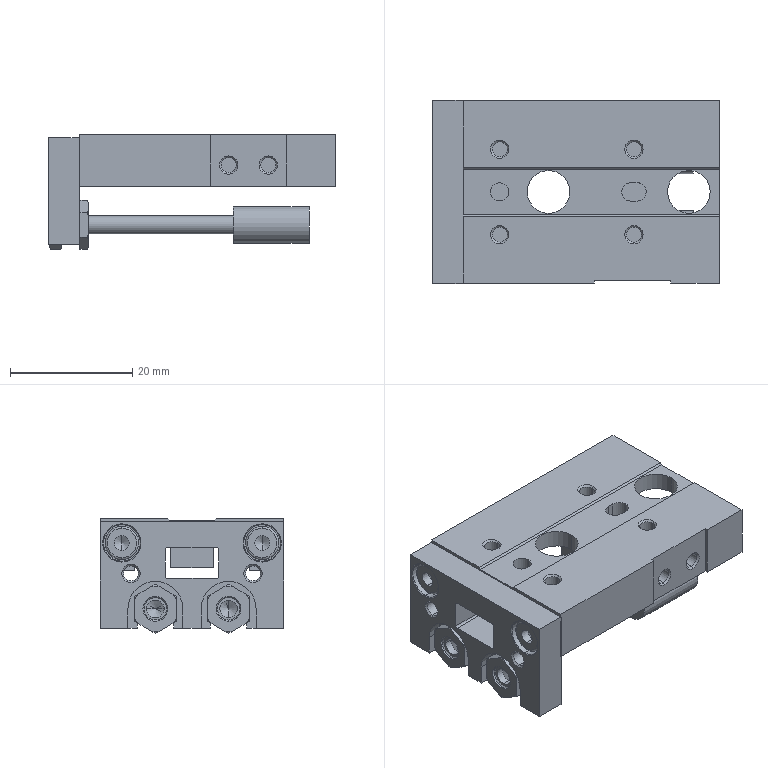Part | STEP file | 11-HLQL6X10-S-0-rod-A11 | 1 solid | 290 faces | box 47 x 30 x 18.84 mm | volume 10073 mm3 | plane 107 | cylinder 95 | cone 84 | torus 4 | commonest cylinder face diameters 8.08 x26 2.459 x16 6 x12 3 x9 5.5 x8 0.6 x4